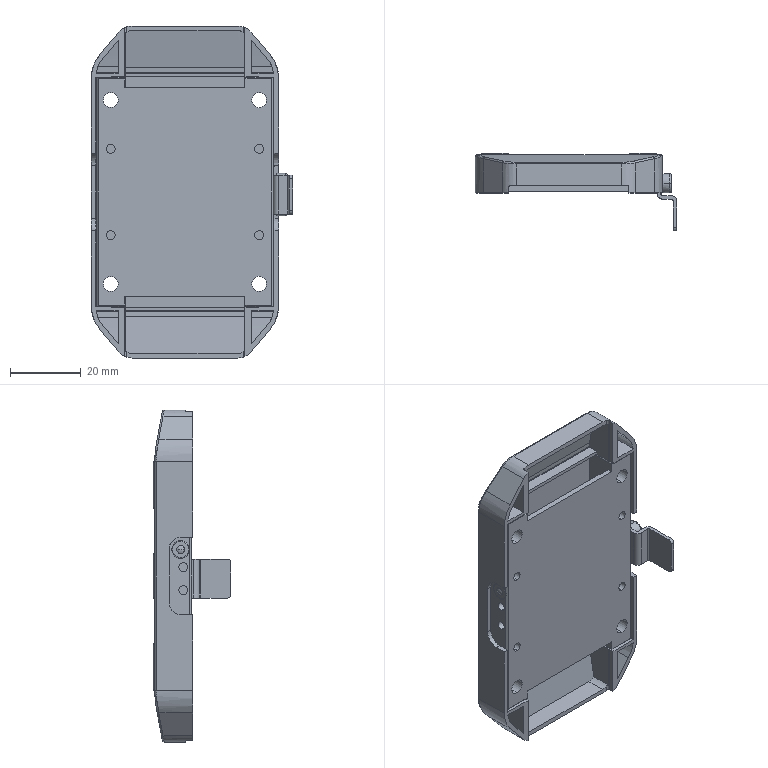Part | SolidWorks | 5 solids | 409 faces | box 57 x 22 x 94 mm | volume 6979 mm3 | plane 177 | cylinder 148 | spline 56 | cone 28 | commonest cylinder face diameters 1 x58 2.5 x16 3.4 x8 4.2 x8 5.54 x8 3 x6